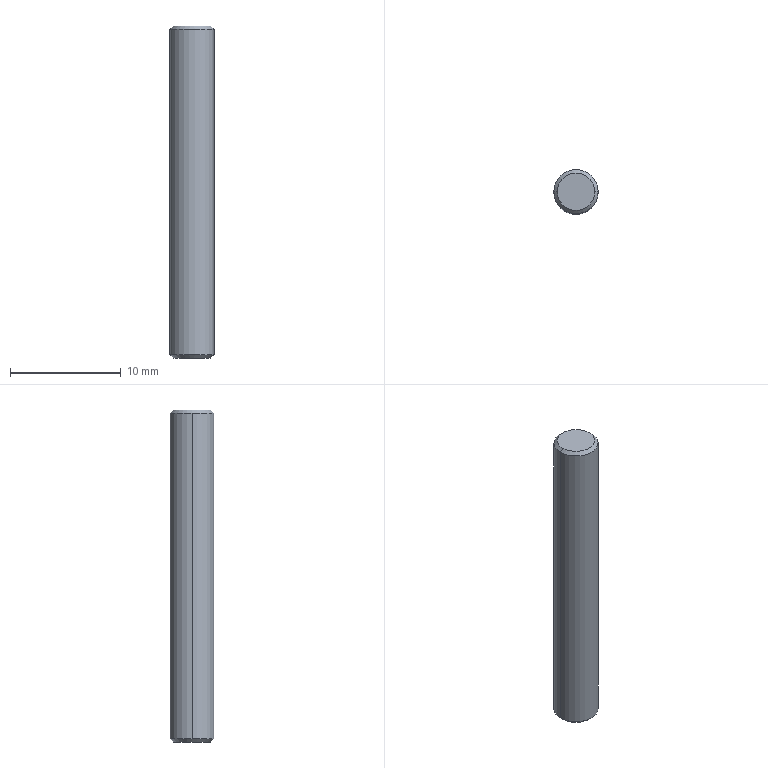Part | NX | features BREP 1 | 1 solid | 8 faces | box 4 x 4 x 30 mm | volume 375.917 mm3 | cone 4 | plane 2 | cylinder 2 | commonest cylinder face diameters 4 x2
STEP:
#1=CARTESIAN_POINT('',(1.7,0.,30.));
#2=VERTEX_POINT('',#1);
#3=CARTESIAN_POINT('',(2.,0.,29.7));
#4=VERTEX_POINT('',#3);
#5=CARTESIAN_POINT('',(1.7,0.,30.));
#6=DIRECTION('',(0.7071,0.,-0.7071));
#7=VECTOR('',#6,1000.);
#8=LINE('',#5,#7);
#9=EDGE_CURVE('',#2,#4,#8,.T.);
#10=ORIENTED_EDGE('',*,*,#9,.F.);
#11=CARTESIAN_POINT('',(-1.7,0.,30.));
#12=VERTEX_POINT('',#11);
#13=CARTESIAN_POINT('',(0.,0.,30.));
#14=DIRECTION('',(0.,0.,1.));
#15=DIRECTION('',(1.,0.,0.));
#16=AXIS2_PLACEMENT_3D('',#13,#14,#15);
#17=CIRCLE('',#16,1.7);
#18=EDGE_CURVE('',#12,#2,#17,.T.);
#19=ORIENTED_EDGE('',*,*,#18,.F.);
#20=CARTESIAN_POINT('',(-2.,0.,29.7));
#21=VERTEX_POINT('',#20);
#22=CARTESIAN_POINT('',(-1.7,0.,30.));
#23=DIRECTION('',(-0.7071,0.,-0.7071));
#24=VECTOR('',#23,1000.);
#25=LINE('',#22,#24);
#26=EDGE_CURVE('',#12,#21,#25,.T.);
#27=ORIENTED_EDGE('',*,*,#26,.T.);
#28=CARTESIAN_POINT('',(0.,0.,29.7));
#29=DIRECTION('',(0.,0.,-1.));
#30=DIRECTION('',(1.,0.,0.));
#31=AXIS2_PLACEMENT_3D('',#28,#29,#30);
#32=CIRCLE('',#31,2.);
#33=EDGE_CURVE('',#4,#21,#32,.T.);
#34=ORIENTED_EDGE('',*,*,#33,.F.);
#35=EDGE_LOOP('',(#10,#19,#27,#34));
#36=FACE_BOUND('',#35,.T.);
#37=CARTESIAN_POINT('',(0.,0.,30.));
#38=DIRECTION('',(0.,0.,-1.));
#39=DIRECTION('',(-1.,0.,0.));
#40=AXIS2_PLACEMENT_3D('',#37,#38,#39);
#41=CONICAL_SURFACE('',#40,1.7,0.7854);
#42=ADVANCED_FACE('',(#36),#41,.T.);
#43=CARTESIAN_POINT('',(-2.,0.,0.3));
#44=VERTEX_POINT('',#43);
#45=CARTESIAN_POINT('',(-1.7,0.,0.));
#46=VERTEX_POINT('',#45);
#47=CARTESIAN_POINT('',(-2.,0.,0.3));
#48=DIRECTION('',(-0.7071,0.,0.7071));
#49=VECTOR('',#48,1000.);
#50=LINE('',#47,#49);
#51=EDGE_CURVE('',#44,#46,#50,.F.);
#52=ORIENTED_EDGE('',*,*,#51,.T.);
#53=CARTESIAN_POINT('',(1.7,0.,0.));
#54=VERTEX_POINT('',#53);
#55=CARTESIAN_POINT('',(0.,0.,0.));
#56=DIRECTION('',(0.,0.,-1.));
#57=DIRECTION('',(1.,0.,0.));
#58=AXIS2_PLACEMENT_3D('',#55,#56,#57);
#59=CIRCLE('',#58,1.7);
#60=EDGE_CURVE('',#54,#46,#59,.T.);
#61=ORIENTED_EDGE('',*,*,#60,.F.);
#62=CARTESIAN_POINT('',(2.,0.,0.3));
#63=VERTEX_POINT('',#62);
#64=CARTESIAN_POINT('',(2.,0.,0.3));
#65=DIRECTION('',(0.7071,0.,0.7071));
#66=VECTOR('',#65,1000.);
#67=LINE('',#64,#66);
#68=EDGE_CURVE('',#63,#54,#67,.F.);
#69=ORIENTED_EDGE('',*,*,#68,.F.);
#70=CARTESIAN_POINT('',(0.,0.,0.3));
#71=DIRECTION('',(0.,0.,1.));
#72=DIRECTION('',(1.,0.,0.));
#73=AXIS2_PLACEMENT_3D('',#70,#71,#72);
#74=CIRCLE('',#73,2.);
#75=EDGE_CURVE('',#44,#63,#74,.T.);
#76=ORIENTED_EDGE('',*,*,#75,.F.);
#77=EDGE_LOOP('',(#52,#61,#69,#76));
#78=FACE_BOUND('',#77,.T.);
#79=CARTESIAN_POINT('',(0.,0.,0.3));
#80=DIRECTION('',(0.,0.,1.));
#81=DIRECTION('',(1.,0.,0.));
#82=AXIS2_PLACEMENT_3D('',#79,#80,#81);
#83=CONICAL_SURFACE('',#82,2.,0.7854);
#84=ADVANCED_FACE('',(#78),#83,.T.);
#85=ORIENTED_EDGE('',*,*,#60,.T.);
#86=CARTESIAN_POINT('',(0.,0.,0.));
#87=DIRECTION('',(0.,0.,-1.));
#88=DIRECTION('',(1.,0.,0.));
#89=AXIS2_PLACEMENT_3D('',#86,#87,#88);
#90=CIRCLE('',#89,1.7);
#91=EDGE_CURVE('',#46,#54,#90,.T.);
#92=ORIENTED_EDGE('',*,*,#91,.T.);
#93=EDGE_LOOP('',(#85,#92));
#94=FACE_BOUND('',#93,.T.);
#95=CARTESIAN_POINT('',(0.,0.,0.));
#96=DIRECTION('',(0.,0.,1.));
#97=DIRECTION('',(1.,0.,0.));
#98=AXIS2_PLACEMENT_3D('',#95,#96,#97);
#99=PLANE('',#98);
#100=ADVANCED_FACE('',(#94),#99,.F.);
#101=ORIENTED_EDGE('',*,*,#18,.T.);
#102=CARTESIAN_POINT('',(0.,0.,30.));
#103=DIRECTION('',(0.,0.,1.));
#104=DIRECTION('',(1.,0.,0.));
#105=AXIS2_PLACEMENT_3D('',#102,#103,#104);
#106=CIRCLE('',#105,1.7);
#107=EDGE_CURVE('',#2,#12,#106,.T.);
#108=ORIENTED_EDGE('',*,*,#107,.T.);
#109=EDGE_LOOP('',(#101,#108));
#110=FACE_BOUND('',#109,.T.);
#111=CARTESIAN_POINT('',(0.,0.,30.));
#112=DIRECTION('',(0.,0.,1.));
#113=DIRECTION('',(1.,0.,0.));
#114=AXIS2_PLACEMENT_3D('',#111,#112,#113);
#115=PLANE('',#114);
#116=ADVANCED_FACE('',(#110),#115,.T.);
#117=CARTESIAN_POINT('',(2.,0.,30.));
#118=DIRECTION('',(0.,0.,-1.));
#119=VECTOR('',#118,1000.);
#120=LINE('',#117,#119);
#121=EDGE_CURVE('',#4,#63,#120,.T.);
#122=ORIENTED_EDGE('',*,*,#121,.F.);
#123=ORIENTED_EDGE('',*,*,#33,.T.);
#124=CARTESIAN_POINT('',(-2.,0.,30.));
#125=DIRECTION('',(0.,0.,-1.));
#126=VECTOR('',#125,1000.);
#127=LINE('',#124,#126);
#128=EDGE_CURVE('',#21,#44,#127,.T.);
#129=ORIENTED_EDGE('',*,*,#128,.T.);
#130=ORIENTED_EDGE('',*,*,#75,.T.);
#131=EDGE_LOOP('',(#122,#123,#129,#130));
#132=FACE_BOUND('',#131,.T.);
#133=CARTESIAN_POINT('',(0.,0.,30.));
#134=DIRECTION('',(0.,0.,-1.));
#135=DIRECTION('',(-1.,0.,0.));
#136=AXIS2_PLACEMENT_3D('',#133,#134,#135);
#137=CYLINDRICAL_SURFACE('',#136,2.);
#138=ADVANCED_FACE('',(#132),#137,.T.);
#139=CARTESIAN_POINT('',(0.,0.,29.7));
#140=DIRECTION('',(0.,0.,-1.));
#141=DIRECTION('',(1.,0.,0.));
#142=AXIS2_PLACEMENT_3D('',#139,#140,#141);
#143=CIRCLE('',#142,2.);
#144=EDGE_CURVE('',#21,#4,#143,.T.);
#145=ORIENTED_EDGE('',*,*,#144,.T.);
#146=ORIENTED_EDGE('',*,*,#121,.T.);
#147=CARTESIAN_POINT('',(0.,0.,0.3));
#148=DIRECTION('',(0.,0.,1.));
#149=DIRECTION('',(1.,0.,0.));
#150=AXIS2_PLACEMENT_3D('',#147,#148,#149);
#151=CIRCLE('',#150,2.);
#152=EDGE_CURVE('',#63,#44,#151,.T.);
#153=ORIENTED_EDGE('',*,*,#152,.T.);
#154=ORIENTED_EDGE('',*,*,#128,.F.);
#155=EDGE_LOOP('',(#145,#146,#153,#154));
#156=FACE_BOUND('',#155,.T.);
#157=CARTESIAN_POINT('',(0.,0.,30.));
#158=DIRECTION('',(0.,0.,-1.));
#159=DIRECTION('',(-1.,0.,0.));
#160=AXIS2_PLACEMENT_3D('',#157,#158,#159);
#161=CYLINDRICAL_SURFACE('',#160,2.);
#162=ADVANCED_FACE('',(#156),#161,.T.);
#163=ORIENTED_EDGE('',*,*,#91,.F.);
#164=ORIENTED_EDGE('',*,*,#51,.F.);
#165=ORIENTED_EDGE('',*,*,#152,.F.);
#166=ORIENTED_EDGE('',*,*,#68,.T.);
#167=EDGE_LOOP('',(#163,#164,#165,#166));
#168=FACE_BOUND('',#167,.T.);
#169=CARTESIAN_POINT('',(0.,0.,0.3));
#170=DIRECTION('',(0.,0.,1.));
#171=DIRECTION('',(1.,0.,0.));
#172=AXIS2_PLACEMENT_3D('',#169,#170,#171);
#173=CONICAL_SURFACE('',#172,2.,0.7854);
#174=ADVANCED_FACE('',(#168),#173,.T.);
#175=ORIENTED_EDGE('',*,*,#107,.F.);
#176=ORIENTED_EDGE('',*,*,#9,.T.);
#177=ORIENTED_EDGE('',*,*,#144,.F.);
#178=ORIENTED_EDGE('',*,*,#26,.F.);
#179=EDGE_LOOP('',(#175,#176,#177,#178));
#180=FACE_BOUND('',#179,.T.);
#181=CARTESIAN_POINT('',(0.,0.,30.));
#182=DIRECTION('',(0.,0.,-1.));
#183=DIRECTION('',(-1.,0.,0.));
#184=AXIS2_PLACEMENT_3D('',#181,#182,#183);
#185=CONICAL_SURFACE('',#184,1.7,0.7854);
#186=ADVANCED_FACE('',(#180),#185,.T.);
#187=CLOSED_SHELL('',(#42,#84,#100,#116,#138,#162,#174,#186));
#188=MANIFOLD_SOLID_BREP('',#187);
#189=(LENGTH_UNIT()NAMED_UNIT(*)SI_UNIT(.MILLI.,.METRE.));
#190=UNCERTAINTY_MEASURE_WITH_UNIT(LENGTH_MEASURE(0.00001),#189,'','');
#191=(NAMED_UNIT(*)PLANE_ANGLE_UNIT()SI_UNIT($,.RADIAN.));
#192=(NAMED_UNIT(*)SI_UNIT($,.STERADIAN.)SOLID_ANGLE_UNIT());
#193=(GEOMETRIC_REPRESENTATION_CONTEXT(3)GLOBAL_UNCERTAINTY_ASSIGNED_CONTEXT((#190))GLOBAL_UNIT_ASSIGNED_CONTEXT((#189,#191,#192))REPRESENTATION_CONTEXT('',''));
#194=ADVANCED_BREP_SHAPE_REPRESENTATION('',(#188),#193);